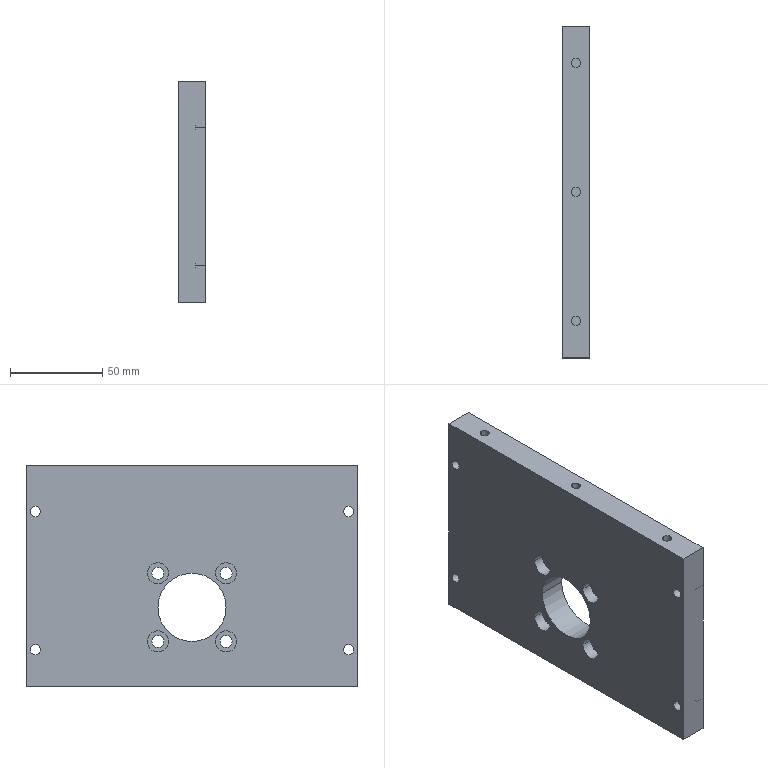Part | STEP file | PN_0005 | 1 solid | 57 faces | box 15 x 180 x 120 mm | volume 300704 mm3 | cylinder 40 | plane 17 | commonest cylinder face diameters 5.5 x8 6.5 x8 9 x8 11.5 x8 5 x6 37 x2